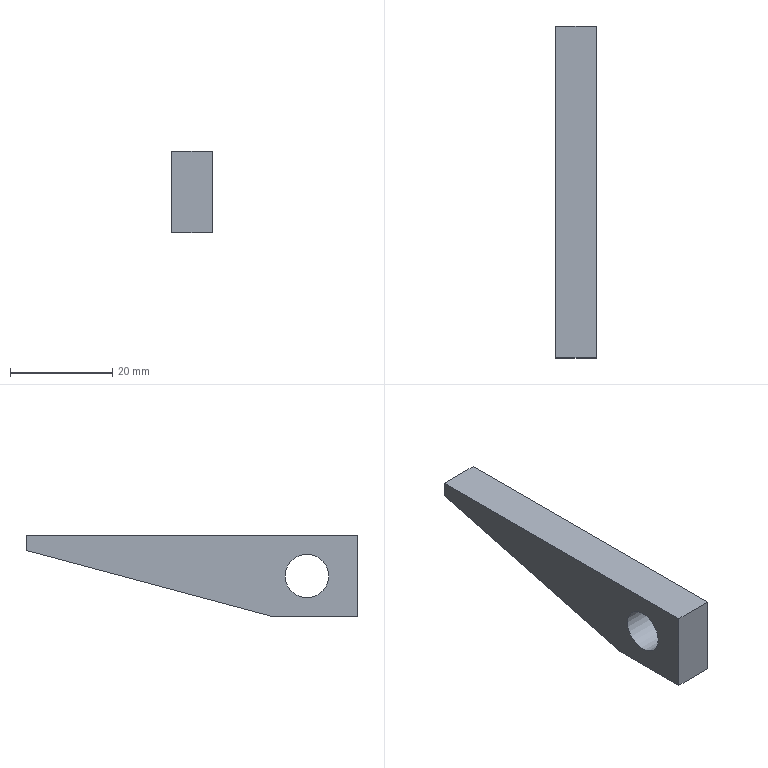Part | NX | features solid 2 | 1 solid | 8 faces | box 8 x 65 x 16 mm | volume 5343 mm3 | plane 7 | cylinder 1 | commonest cylinder face diameters 8.5 x1
STEP:
#1=CARTESIAN_POINT('',(-681.,-480.,-105.));
#2=VERTEX_POINT('',#1);
#3=CARTESIAN_POINT('',(-681.,-463.517,-105.));
#4=VERTEX_POINT('',#3);
#5=CARTESIAN_POINT('',(-681.,-480.,-105.));
#6=DIRECTION('',(0.,1.,0.));
#7=VECTOR('',#6,1000.);
#8=LINE('',#5,#7);
#9=EDGE_CURVE('',#2,#4,#8,.T.);
#10=ORIENTED_EDGE('',*,*,#9,.F.);
#11=CARTESIAN_POINT('',(-689.,-480.,-105.));
#12=VERTEX_POINT('',#11);
#13=CARTESIAN_POINT('',(-681.,-480.,-105.));
#14=DIRECTION('',(-1.,0.,0.));
#15=VECTOR('',#14,1000.);
#16=LINE('',#13,#15);
#17=EDGE_CURVE('',#2,#12,#16,.T.);
#18=ORIENTED_EDGE('',*,*,#17,.T.);
#19=CARTESIAN_POINT('',(-689.,-463.517,-105.));
#20=VERTEX_POINT('',#19);
#21=CARTESIAN_POINT('',(-689.,-480.,-105.));
#22=DIRECTION('',(0.,1.,0.));
#23=VECTOR('',#22,1000.);
#24=LINE('',#21,#23);
#25=EDGE_CURVE('',#12,#20,#24,.T.);
#26=ORIENTED_EDGE('',*,*,#25,.T.);
#27=CARTESIAN_POINT('',(-681.,-463.517,-105.));
#28=DIRECTION('',(-1.,0.,0.));
#29=VECTOR('',#28,1000.);
#30=LINE('',#27,#29);
#31=EDGE_CURVE('',#4,#20,#30,.T.);
#32=ORIENTED_EDGE('',*,*,#31,.F.);
#33=EDGE_LOOP('',(#10,#18,#26,#32));
#34=FACE_BOUND('',#33,.T.);
#35=CARTESIAN_POINT('',(-681.,-480.,-105.));
#36=DIRECTION('',(0.,0.,-1.));
#37=DIRECTION('',(0.,-1.,0.));
#38=AXIS2_PLACEMENT_3D('',#35,#36,#37);
#39=PLANE('',#38);
#40=ADVANCED_FACE('',(#34),#39,.T.);
#41=CARTESIAN_POINT('',(-689.,-415.,-92.));
#42=VERTEX_POINT('',#41);
#43=CARTESIAN_POINT('',(-689.,-415.,-89.));
#44=VERTEX_POINT('',#43);
#45=CARTESIAN_POINT('',(-689.,-415.,-105.));
#46=DIRECTION('',(0.,0.,1.));
#47=VECTOR('',#46,1000.);
#48=LINE('',#45,#47);
#49=EDGE_CURVE('',#42,#44,#48,.T.);
#50=ORIENTED_EDGE('',*,*,#49,.T.);
#51=CARTESIAN_POINT('',(-681.,-415.,-89.));
#52=VERTEX_POINT('',#51);
#53=CARTESIAN_POINT('',(-681.,-415.,-89.));
#54=DIRECTION('',(-1.,0.,0.));
#55=VECTOR('',#54,1000.);
#56=LINE('',#53,#55);
#57=EDGE_CURVE('',#52,#44,#56,.T.);
#58=ORIENTED_EDGE('',*,*,#57,.F.);
#59=CARTESIAN_POINT('',(-681.,-415.,-92.));
#60=VERTEX_POINT('',#59);
#61=CARTESIAN_POINT('',(-681.,-415.,-105.));
#62=DIRECTION('',(0.,0.,1.));
#63=VECTOR('',#62,1000.);
#64=LINE('',#61,#63);
#65=EDGE_CURVE('',#60,#52,#64,.T.);
#66=ORIENTED_EDGE('',*,*,#65,.F.);
#67=CARTESIAN_POINT('',(-681.,-415.,-92.));
#68=DIRECTION('',(1.,0.,0.));
#69=VECTOR('',#68,1000.);
#70=LINE('',#67,#69);
#71=EDGE_CURVE('',#42,#60,#70,.T.);
#72=ORIENTED_EDGE('',*,*,#71,.F.);
#73=EDGE_LOOP('',(#50,#58,#66,#72));
#74=FACE_BOUND('',#73,.T.);
#75=CARTESIAN_POINT('',(-681.,-415.,-105.));
#76=DIRECTION('',(0.,1.,0.));
#77=DIRECTION('',(0.,0.,-1.));
#78=AXIS2_PLACEMENT_3D('',#75,#76,#77);
#79=PLANE('',#78);
#80=ADVANCED_FACE('',(#74),#79,.T.);
#81=CARTESIAN_POINT('',(-689.,-480.,-89.));
#82=VERTEX_POINT('',#81);
#83=CARTESIAN_POINT('',(-689.,-415.,-89.));
#84=DIRECTION('',(0.,-1.,0.));
#85=VECTOR('',#84,1000.);
#86=LINE('',#83,#85);
#87=EDGE_CURVE('',#44,#82,#86,.T.);
#88=ORIENTED_EDGE('',*,*,#87,.T.);
#89=CARTESIAN_POINT('',(-681.,-480.,-89.));
#90=VERTEX_POINT('',#89);
#91=CARTESIAN_POINT('',(-681.,-480.,-89.));
#92=DIRECTION('',(-1.,0.,0.));
#93=VECTOR('',#92,1000.);
#94=LINE('',#91,#93);
#95=EDGE_CURVE('',#90,#82,#94,.T.);
#96=ORIENTED_EDGE('',*,*,#95,.F.);
#97=CARTESIAN_POINT('',(-681.,-415.,-89.));
#98=DIRECTION('',(0.,-1.,0.));
#99=VECTOR('',#98,1000.);
#100=LINE('',#97,#99);
#101=EDGE_CURVE('',#52,#90,#100,.T.);
#102=ORIENTED_EDGE('',*,*,#101,.F.);
#103=ORIENTED_EDGE('',*,*,#57,.T.);
#104=EDGE_LOOP('',(#88,#96,#102,#103));
#105=FACE_BOUND('',#104,.T.);
#106=CARTESIAN_POINT('',(-681.,-415.,-89.));
#107=DIRECTION('',(0.,0.,1.));
#108=DIRECTION('',(1.,0.,0.));
#109=AXIS2_PLACEMENT_3D('',#106,#107,#108);
#110=PLANE('',#109);
#111=ADVANCED_FACE('',(#105),#110,.T.);
#112=CARTESIAN_POINT('',(-689.,-480.,-89.));
#113=DIRECTION('',(0.,0.,-1.));
#114=VECTOR('',#113,1000.);
#115=LINE('',#112,#114);
#116=EDGE_CURVE('',#82,#12,#115,.T.);
#117=ORIENTED_EDGE('',*,*,#116,.T.);
#118=ORIENTED_EDGE('',*,*,#17,.F.);
#119=CARTESIAN_POINT('',(-681.,-480.,-89.));
#120=DIRECTION('',(0.,0.,-1.));
#121=VECTOR('',#120,1000.);
#122=LINE('',#119,#121);
#123=EDGE_CURVE('',#90,#2,#122,.T.);
#124=ORIENTED_EDGE('',*,*,#123,.F.);
#125=ORIENTED_EDGE('',*,*,#95,.T.);
#126=EDGE_LOOP('',(#117,#118,#124,#125));
#127=FACE_BOUND('',#126,.T.);
#128=CARTESIAN_POINT('',(-681.,-480.,-89.));
#129=DIRECTION('',(0.,-1.,0.));
#130=DIRECTION('',(0.,0.,1.));
#131=AXIS2_PLACEMENT_3D('',#128,#129,#130);
#132=PLANE('',#131);
#133=ADVANCED_FACE('',(#127),#132,.T.);
#134=CARTESIAN_POINT('',(-681.,-474.25,-97.));
#135=VERTEX_POINT('',#134);
#136=CARTESIAN_POINT('',(-681.,-470.,-97.));
#137=DIRECTION('',(-1.,0.,0.));
#138=DIRECTION('',(0.,-1.,0.));
#139=AXIS2_PLACEMENT_3D('',#136,#137,#138);
#140=CIRCLE('',#139,4.25);
#141=EDGE_CURVE('',#135,#135,#140,.T.);
#142=ORIENTED_EDGE('',*,*,#141,.F.);
#143=EDGE_LOOP('',(#142));
#144=FACE_BOUND('',#143,.T.);
#145=CARTESIAN_POINT('',(-689.,-474.25,-97.));
#146=VERTEX_POINT('',#145);
#147=CARTESIAN_POINT('',(-689.,-470.,-97.));
#148=DIRECTION('',(-1.,0.,0.));
#149=DIRECTION('',(0.,-1.,0.));
#150=AXIS2_PLACEMENT_3D('',#147,#148,#149);
#151=CIRCLE('',#150,4.25);
#152=EDGE_CURVE('',#146,#146,#151,.T.);
#153=ORIENTED_EDGE('',*,*,#152,.T.);
#154=EDGE_LOOP('',(#153));
#155=FACE_BOUND('',#154,.T.);
#156=CARTESIAN_POINT('',(-681.,-470.,-97.));
#157=DIRECTION('',(-1.,0.,0.));
#158=DIRECTION('',(0.,0.,1.));
#159=AXIS2_PLACEMENT_3D('',#156,#157,#158);
#160=CYLINDRICAL_SURFACE('',#159,4.25);
#161=ADVANCED_FACE('',(#144,#155),#160,.F.);
#162=ORIENTED_EDGE('',*,*,#65,.T.);
#163=ORIENTED_EDGE('',*,*,#101,.T.);
#164=ORIENTED_EDGE('',*,*,#123,.T.);
#165=ORIENTED_EDGE('',*,*,#9,.T.);
#166=CARTESIAN_POINT('',(-681.,-478.896,-109.121));
#167=DIRECTION('',(0.,0.9659,0.2588));
#168=VECTOR('',#167,1000.);
#169=LINE('',#166,#168);
#170=EDGE_CURVE('',#60,#4,#169,.F.);
#171=ORIENTED_EDGE('',*,*,#170,.F.);
#172=EDGE_LOOP('',(#162,#163,#164,#165,#171));
#173=FACE_BOUND('',#172,.T.);
#174=ORIENTED_EDGE('',*,*,#141,.T.);
#175=EDGE_LOOP('',(#174));
#176=FACE_BOUND('',#175,.T.);
#177=CARTESIAN_POINT('',(-681.,-480.,-105.));
#178=DIRECTION('',(1.,0.,0.));
#179=DIRECTION('',(0.,0.,-1.));
#180=AXIS2_PLACEMENT_3D('',#177,#178,#179);
#181=PLANE('',#180);
#182=ADVANCED_FACE('',(#173,#176),#181,.T.);
#183=ORIENTED_EDGE('',*,*,#25,.F.);
#184=ORIENTED_EDGE('',*,*,#116,.F.);
#185=ORIENTED_EDGE('',*,*,#87,.F.);
#186=ORIENTED_EDGE('',*,*,#49,.F.);
#187=CARTESIAN_POINT('',(-689.,-463.517,-105.));
#188=DIRECTION('',(0.,-0.9659,-0.2588));
#189=VECTOR('',#188,1000.);
#190=LINE('',#187,#189);
#191=EDGE_CURVE('',#20,#42,#190,.F.);
#192=ORIENTED_EDGE('',*,*,#191,.F.);
#193=EDGE_LOOP('',(#183,#184,#185,#186,#192));
#194=FACE_BOUND('',#193,.T.);
#195=ORIENTED_EDGE('',*,*,#152,.F.);
#196=EDGE_LOOP('',(#195));
#197=FACE_BOUND('',#196,.T.);
#198=CARTESIAN_POINT('',(-689.,-480.,-105.));
#199=DIRECTION('',(1.,0.,0.));
#200=DIRECTION('',(0.,0.,-1.));
#201=AXIS2_PLACEMENT_3D('',#198,#199,#200);
#202=PLANE('',#201);
#203=ADVANCED_FACE('',(#194,#197),#202,.F.);
#204=ORIENTED_EDGE('',*,*,#170,.T.);
#205=ORIENTED_EDGE('',*,*,#31,.T.);
#206=ORIENTED_EDGE('',*,*,#191,.T.);
#207=ORIENTED_EDGE('',*,*,#71,.T.);
#208=EDGE_LOOP('',(#204,#205,#206,#207));
#209=FACE_BOUND('',#208,.T.);
#210=CARTESIAN_POINT('',(-681.,-463.517,-105.));
#211=DIRECTION('',(0.,-0.2588,0.9659));
#212=DIRECTION('',(0.,0.9659,0.2588));
#213=AXIS2_PLACEMENT_3D('',#210,#211,#212);
#214=PLANE('',#213);
#215=ADVANCED_FACE('',(#209),#214,.F.);
#216=CLOSED_SHELL('',(#40,#80,#111,#133,#161,#182,#203,#215));
#217=MANIFOLD_SOLID_BREP('',#216);
#218=(LENGTH_UNIT()NAMED_UNIT(*)SI_UNIT(.MILLI.,.METRE.));
#219=UNCERTAINTY_MEASURE_WITH_UNIT(LENGTH_MEASURE(0.00001),#218,'','');
#220=(NAMED_UNIT(*)PLANE_ANGLE_UNIT()SI_UNIT($,.RADIAN.));
#221=(NAMED_UNIT(*)SI_UNIT($,.STERADIAN.)SOLID_ANGLE_UNIT());
#222=(GEOMETRIC_REPRESENTATION_CONTEXT(3)GLOBAL_UNCERTAINTY_ASSIGNED_CONTEXT((#219))GLOBAL_UNIT_ASSIGNED_CONTEXT((#218,#220,#221))REPRESENTATION_CONTEXT('',''));
#223=ADVANCED_BREP_SHAPE_REPRESENTATION('',(#217),#222);